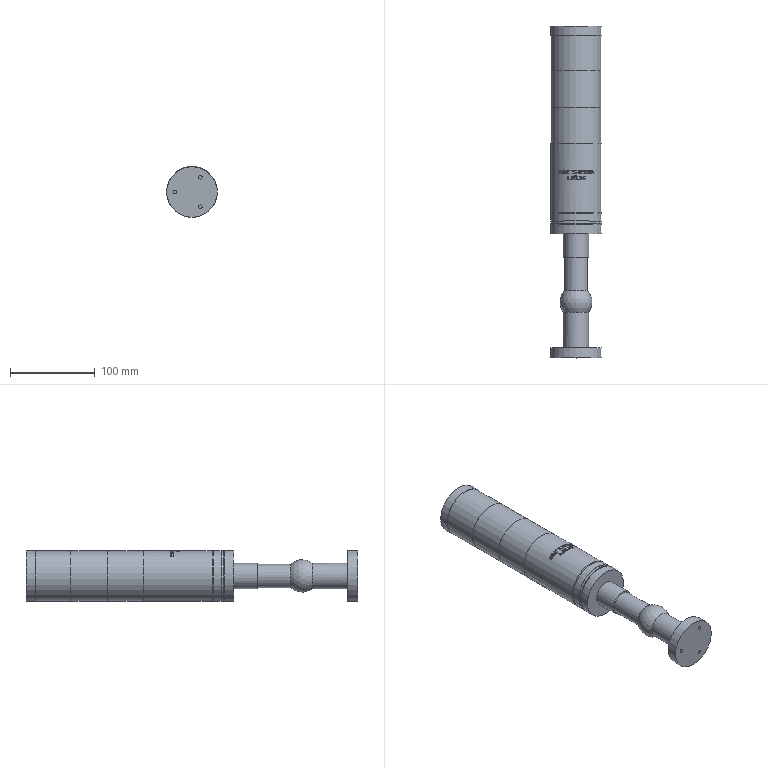Part | NX | 1 solid | 387 faces | box 60 x 391.5 x 60 mm | volume 807743 mm3 | spline 165 | plane 160 | cylinder 61 | sphere 1 | commonest cylinder face diameters 59.9 x31 59.7 x14 4.3 x3 11.3 x3 30 x2 59 x2